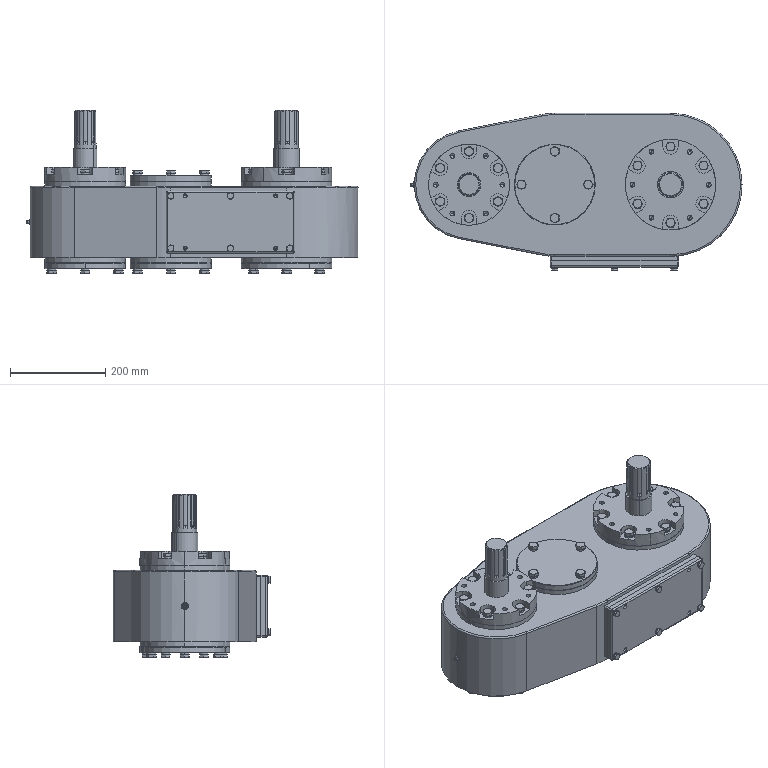Part | SolidWorks | features ReferencePattern 66, LocalCirPattern 6, LocalLPattern 2, CompositeCurve 1, MirrorCompFeat 1 | 105 solids | 4483 faces | volume 19308799 mm3 | cylinder 1246 | plane 1195 | cone 814 | sphere 644 | torus 448 | spline 136 | commonest cylinder face diameters 12.2 x90 18.367 x90 10.2 x84 12 x60 12.5 x60 18 x60